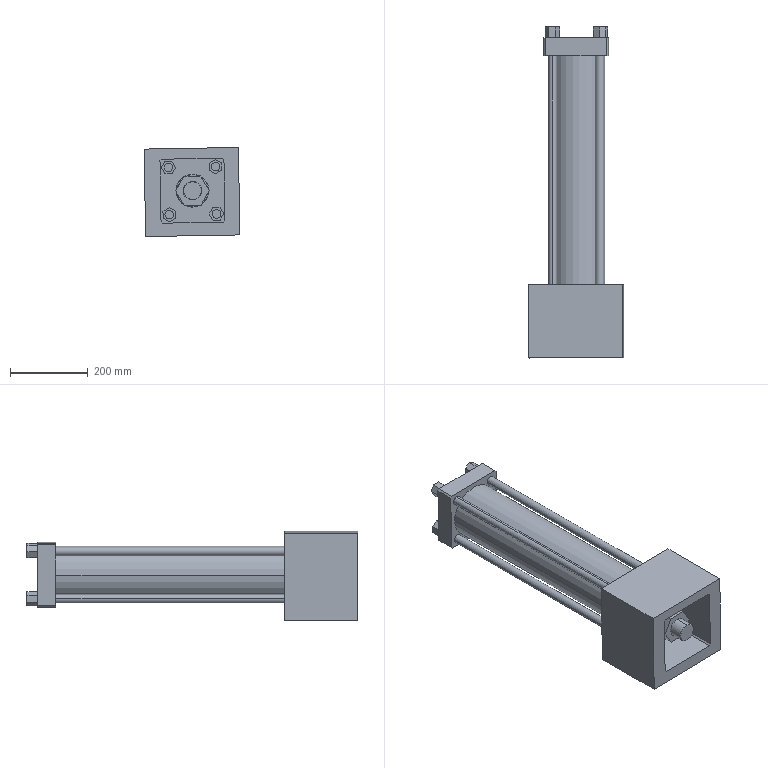Part | STEP file | 2026.6.15-Main Assembly图.sldasm-Part-32 | 1 solid | 175 faces | box 247.048 x 856 x 229.797 mm | volume 19267675 mm3 | plane 123 | cylinder 36 | cone 16 | commonest cylinder face diameters 22 x24 23 x4 48 x2 60 x2 85 x2 140 x2